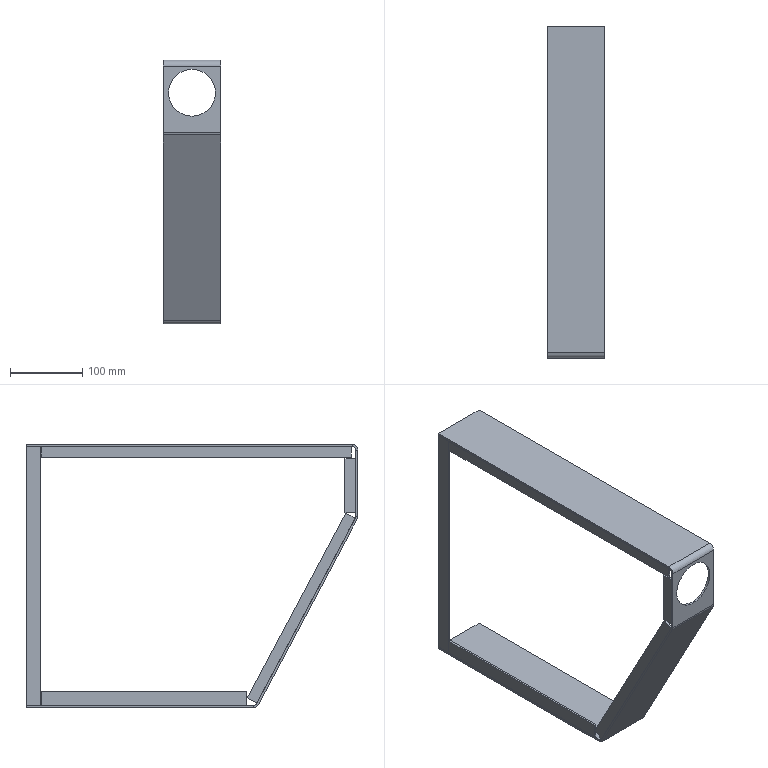Part | SolidWorks | features ICE 3, FlatPattern 1, SMBaseFlange 1, SheetMetal 1 | 6 solids | 62 faces | box 80 x 460 x 365 mm | volume 345434 mm3 | plane 54 | cylinder 8 | commonest cylinder face diameters 10 x3 16 x3 65 x2
STEP:
#1=CARTESIAN_POINT('',(40.,3.,-12.5));
#2=VERTEX_POINT('',#1);
#3=CARTESIAN_POINT('',(40.,3.,-77.5));
#4=VERTEX_POINT('',#3);
#5=CARTESIAN_POINT('',(40.,3.,-45.));
#6=DIRECTION('',(0.,-1.,0.));
#7=DIRECTION('',(0.,0.,-1.));
#8=AXIS2_PLACEMENT_3D('',#5,#6,#7);
#9=CIRCLE('',#8,32.5);
#10=EDGE_CURVE('',#2,#4,#9,.T.);
#11=ORIENTED_EDGE('',*,*,#10,.F.);
#12=CARTESIAN_POINT('',(40.,0.,-12.5));
#13=VERTEX_POINT('',#12);
#14=CARTESIAN_POINT('',(40.,10.,-12.5));
#15=DIRECTION('',(0.,-1.,0.));
#16=VECTOR('',#15,1000.);
#17=LINE('',#14,#16);
#18=EDGE_CURVE('',#2,#13,#17,.T.);
#19=ORIENTED_EDGE('',*,*,#18,.T.);
#20=CARTESIAN_POINT('',(40.,0.,-77.5));
#21=VERTEX_POINT('',#20);
#22=CARTESIAN_POINT('',(40.,0.,-45.));
#23=DIRECTION('',(0.,-1.,0.));
#24=DIRECTION('',(0.,0.,-1.));
#25=AXIS2_PLACEMENT_3D('',#22,#23,#24);
#26=CIRCLE('',#25,32.5);
#27=EDGE_CURVE('',#13,#21,#26,.T.);
#28=ORIENTED_EDGE('',*,*,#27,.T.);
#29=CARTESIAN_POINT('',(40.,10.,-77.5));
#30=DIRECTION('',(0.,-1.,0.));
#31=VECTOR('',#30,1000.);
#32=LINE('',#29,#31);
#33=EDGE_CURVE('',#4,#21,#32,.T.);
#34=ORIENTED_EDGE('',*,*,#33,.F.);
#35=EDGE_LOOP('',(#11,#19,#28,#34));
#36=FACE_OUTER_BOUND('',#35,.T.);
#37=CARTESIAN_POINT('',(40.,10.,-45.));
#38=DIRECTION('',(0.,-1.,0.));
#39=DIRECTION('',(0.,0.,-1.));
#40=AXIS2_PLACEMENT_3D('',#37,#38,#39);
#41=CYLINDRICAL_SURFACE('',#40,32.5);
#42=ADVANCED_FACE('',(#36),#41,.F.);
#43=CARTESIAN_POINT('',(80.,137.743,-360.756));
#44=VERTEX_POINT('',#43);
#45=CARTESIAN_POINT('',(80.,140.392,-359.347));
#46=VERTEX_POINT('',#45);
#47=CARTESIAN_POINT('',(80.,137.743,-360.756));
#48=DIRECTION('',(0.,0.8829,0.4695));
#49=VECTOR('',#48,1000.);
#50=LINE('',#47,#49);
#51=EDGE_CURVE('',#44,#46,#50,.T.);
#52=ORIENTED_EDGE('',*,*,#51,.F.);
#53=CARTESIAN_POINT('',(80.,144.807,-365.));
#54=VERTEX_POINT('',#53);
#55=CARTESIAN_POINT('',(80.,144.807,-357.));
#56=DIRECTION('',(-1.,0.,0.));
#57=DIRECTION('',(0.,0.,-1.));
#58=AXIS2_PLACEMENT_3D('',#55,#56,#57);
#59=CIRCLE('',#58,8.);
#60=EDGE_CURVE('',#54,#44,#59,.T.);
#61=ORIENTED_EDGE('',*,*,#60,.F.);
#62=CARTESIAN_POINT('',(80.,144.807,-362.));
#63=VERTEX_POINT('',#62);
#64=CARTESIAN_POINT('',(80.,144.807,-362.));
#65=DIRECTION('',(0.,0.,-1.));
#66=VECTOR('',#65,1000.);
#67=LINE('',#64,#66);
#68=EDGE_CURVE('',#63,#54,#67,.T.);
#69=ORIENTED_EDGE('',*,*,#68,.F.);
#70=CARTESIAN_POINT('',(80.,144.807,-357.));
#71=DIRECTION('',(-1.,0.,0.));
#72=DIRECTION('',(0.,0.,-1.));
#73=AXIS2_PLACEMENT_3D('',#70,#71,#72);
#74=CIRCLE('',#73,5.);
#75=EDGE_CURVE('',#63,#46,#74,.T.);
#76=ORIENTED_EDGE('',*,*,#75,.T.);
#77=EDGE_LOOP('',(#52,#61,#69,#76));
#78=FACE_OUTER_BOUND('',#77,.T.);
#79=CARTESIAN_POINT('',(80.,137.743,-360.756));
#80=DIRECTION('',(1.,0.,0.));
#81=DIRECTION('',(0.,0.,-1.));
#82=AXIS2_PLACEMENT_3D('',#79,#80,#81);
#83=PLANE('',#82);
#84=ADVANCED_FACE('',(#78),#83,.T.);
#85=CARTESIAN_POINT('',(80.,0.9364,-103.459));
#86=VERTEX_POINT('',#85);
#87=CARTESIAN_POINT('',(80.,0.,-101.698));
#88=DIRECTION('',(0.,-0.4695,0.8829));
#89=VECTOR('',#88,1000.);
#90=LINE('',#87,#89);
#91=EDGE_CURVE('',#44,#86,#90,.T.);
#92=ORIENTED_EDGE('',*,*,#91,.F.);
#93=ORIENTED_EDGE('',*,*,#51,.T.);
#94=CARTESIAN_POINT('',(80.,3.585,-102.051));
#95=VERTEX_POINT('',#94);
#96=CARTESIAN_POINT('',(80.,2.649,-100.29));
#97=DIRECTION('',(0.,-0.4695,0.8829));
#98=VECTOR('',#97,1000.);
#99=LINE('',#96,#98);
#100=EDGE_CURVE('',#46,#95,#99,.T.);
#101=ORIENTED_EDGE('',*,*,#100,.T.);
#102=CARTESIAN_POINT('',(80.,3.585,-102.051));
#103=DIRECTION('',(0.,-0.8829,-0.4695));
#104=VECTOR('',#103,1000.);
#105=LINE('',#102,#104);
#106=EDGE_CURVE('',#95,#86,#105,.T.);
#107=ORIENTED_EDGE('',*,*,#106,.T.);
#108=EDGE_LOOP('',(#92,#93,#101,#107));
#109=FACE_OUTER_BOUND('',#108,.T.);
#110=CARTESIAN_POINT('',(80.,144.807,-362.));
#111=DIRECTION('',(1.,0.,0.));
#112=DIRECTION('',(0.,0.,-1.));
#113=AXIS2_PLACEMENT_3D('',#110,#111,#112);
#114=PLANE('',#113);
#115=ADVANCED_FACE('',(#109),#114,.T.);
#116=CARTESIAN_POINT('',(0.,144.807,-365.));
#117=VERTEX_POINT('',#116);
#118=CARTESIAN_POINT('',(0.,144.807,-362.));
#119=VERTEX_POINT('',#118);
#120=CARTESIAN_POINT('',(0.,144.807,-365.));
#121=DIRECTION('',(0.,0.,1.));
#122=VECTOR('',#121,1000.);
#123=LINE('',#120,#122);
#124=EDGE_CURVE('',#117,#119,#123,.T.);
#125=ORIENTED_EDGE('',*,*,#124,.F.);
#126=CARTESIAN_POINT('',(0.,137.743,-360.756));
#127=VERTEX_POINT('',#126);
#128=CARTESIAN_POINT('',(0.,144.807,-357.));
#129=DIRECTION('',(-1.,0.,0.));
#130=DIRECTION('',(0.,0.,-1.));
#131=AXIS2_PLACEMENT_3D('',#128,#129,#130);
#132=CIRCLE('',#131,8.);
#133=EDGE_CURVE('',#117,#127,#132,.T.);
#134=ORIENTED_EDGE('',*,*,#133,.T.);
#135=CARTESIAN_POINT('',(0.,140.392,-359.347));
#136=VERTEX_POINT('',#135);
#137=CARTESIAN_POINT('',(0.,140.392,-359.347));
#138=DIRECTION('',(0.,-0.8829,-0.4695));
#139=VECTOR('',#138,1000.);
#140=LINE('',#137,#139);
#141=EDGE_CURVE('',#136,#127,#140,.T.);
#142=ORIENTED_EDGE('',*,*,#141,.F.);
#143=CARTESIAN_POINT('',(0.,144.807,-357.));
#144=DIRECTION('',(-1.,0.,0.));
#145=DIRECTION('',(0.,0.,-1.));
#146=AXIS2_PLACEMENT_3D('',#143,#144,#145);
#147=CIRCLE('',#146,5.);
#148=EDGE_CURVE('',#119,#136,#147,.T.);
#149=ORIENTED_EDGE('',*,*,#148,.F.);
#150=EDGE_LOOP('',(#125,#134,#142,#149));
#151=FACE_OUTER_BOUND('',#150,.T.);
#152=CARTESIAN_POINT('',(0.,144.807,-365.));
#153=DIRECTION('',(-1.,0.,0.));
#154=DIRECTION('',(0.,0.,1.));
#155=AXIS2_PLACEMENT_3D('',#152,#153,#154);
#156=PLANE('',#155);
#157=ADVANCED_FACE('',(#151),#156,.T.);
#158=CARTESIAN_POINT('',(0.,460.,-365.));
#159=VERTEX_POINT('',#158);
#160=CARTESIAN_POINT('',(0.,140.,-365.));
#161=DIRECTION('',(0.,-1.,0.));
#162=VECTOR('',#161,1000.);
#163=LINE('',#160,#162);
#164=EDGE_CURVE('',#159,#117,#163,.T.);
#165=ORIENTED_EDGE('',*,*,#164,.T.);
#166=ORIENTED_EDGE('',*,*,#124,.T.);
#167=CARTESIAN_POINT('',(0.,460.,-362.));
#168=VERTEX_POINT('',#167);
#169=CARTESIAN_POINT('',(0.,140.,-362.));
#170=DIRECTION('',(0.,-1.,0.));
#171=VECTOR('',#170,1000.);
#172=LINE('',#169,#171);
#173=EDGE_CURVE('',#168,#119,#172,.T.);
#174=ORIENTED_EDGE('',*,*,#173,.F.);
#175=CARTESIAN_POINT('',(0.,460.,-362.));
#176=DIRECTION('',(0.,0.,-1.));
#177=VECTOR('',#176,1000.);
#178=LINE('',#175,#177);
#179=EDGE_CURVE('',#168,#159,#178,.T.);
#180=ORIENTED_EDGE('',*,*,#179,.T.);
#181=EDGE_LOOP('',(#165,#166,#174,#180));
#182=FACE_OUTER_BOUND('',#181,.T.);
#183=CARTESIAN_POINT('',(0.,140.392,-359.347));
#184=DIRECTION('',(-1.,0.,0.));
#185=DIRECTION('',(0.,0.,1.));
#186=AXIS2_PLACEMENT_3D('',#183,#184,#185);
#187=PLANE('',#186);
#188=ADVANCED_FACE('',(#182),#187,.T.);
#189=CARTESIAN_POINT('',(80.,0.,-99.704));
#190=VERTEX_POINT('',#189);
#191=CARTESIAN_POINT('',(80.,3.,-99.704));
#192=VERTEX_POINT('',#191);
#193=CARTESIAN_POINT('',(80.,0.,-99.704));
#194=DIRECTION('',(0.,1.,0.));
#195=VECTOR('',#194,1000.);
#196=LINE('',#193,#195);
#197=EDGE_CURVE('',#190,#192,#196,.T.);
#198=ORIENTED_EDGE('',*,*,#197,.F.);
#199=CARTESIAN_POINT('',(80.,8.,-99.704));
#200=DIRECTION('',(-1.,0.,0.));
#201=DIRECTION('',(0.,0.,-1.));
#202=AXIS2_PLACEMENT_3D('',#199,#200,#201);
#203=CIRCLE('',#202,8.);
#204=EDGE_CURVE('',#86,#190,#203,.T.);
#205=ORIENTED_EDGE('',*,*,#204,.F.);
#206=ORIENTED_EDGE('',*,*,#106,.F.);
#207=CARTESIAN_POINT('',(80.,8.,-99.704));
#208=DIRECTION('',(-1.,0.,0.));
#209=DIRECTION('',(0.,0.,-1.));
#210=AXIS2_PLACEMENT_3D('',#207,#208,#209);
#211=CIRCLE('',#210,5.);
#212=EDGE_CURVE('',#95,#192,#211,.T.);
#213=ORIENTED_EDGE('',*,*,#212,.T.);
#214=EDGE_LOOP('',(#198,#205,#206,#213));
#215=FACE_OUTER_BOUND('',#214,.T.);
#216=CARTESIAN_POINT('',(80.,0.,-99.704));
#217=DIRECTION('',(1.,0.,0.));
#218=DIRECTION('',(0.,0.,-1.));
#219=AXIS2_PLACEMENT_3D('',#216,#217,#218);
#220=PLANE('',#219);
#221=ADVANCED_FACE('',(#215),#220,.T.);
#222=CARTESIAN_POINT('',(80.,0.,-8.));
#223=VERTEX_POINT('',#222);
#224=CARTESIAN_POINT('',(80.,0.,0.));
#225=DIRECTION('',(0.,0.,1.));
#226=VECTOR('',#225,1000.);
#227=LINE('',#224,#226);
#228=EDGE_CURVE('',#190,#223,#227,.T.);
#229=ORIENTED_EDGE('',*,*,#228,.F.);
#230=ORIENTED_EDGE('',*,*,#197,.T.);
#231=CARTESIAN_POINT('',(80.,3.,-8.));
#232=VERTEX_POINT('',#231);
#233=CARTESIAN_POINT('',(80.,3.,0.));
#234=DIRECTION('',(0.,0.,1.));
#235=VECTOR('',#234,1000.);
#236=LINE('',#233,#235);
#237=EDGE_CURVE('',#192,#232,#236,.T.);
#238=ORIENTED_EDGE('',*,*,#237,.T.);
#239=CARTESIAN_POINT('',(80.,3.,-8.));
#240=DIRECTION('',(0.,-1.,0.));
#241=VECTOR('',#240,1000.);
#242=LINE('',#239,#241);
#243=EDGE_CURVE('',#232,#223,#242,.T.);
#244=ORIENTED_EDGE('',*,*,#243,.T.);
#245=EDGE_LOOP('',(#229,#230,#238,#244));
#246=FACE_OUTER_BOUND('',#245,.T.);
#247=CARTESIAN_POINT('',(80.,3.585,-102.051));
#248=DIRECTION('',(1.,0.,0.));
#249=DIRECTION('',(0.,0.,-1.));
#250=AXIS2_PLACEMENT_3D('',#247,#248,#249);
#251=PLANE('',#250);
#252=ADVANCED_FACE('',(#246),#251,.T.);
#253=CARTESIAN_POINT('',(0.,0.9364,-103.459));
#254=VERTEX_POINT('',#253);
#255=CARTESIAN_POINT('',(0.,3.585,-102.051));
#256=VERTEX_POINT('',#255);
#257=CARTESIAN_POINT('',(0.,0.9364,-103.459));
#258=DIRECTION('',(0.,0.8829,0.4695));
#259=VECTOR('',#258,1000.);
#260=LINE('',#257,#259);
#261=EDGE_CURVE('',#254,#256,#260,.T.);
#262=ORIENTED_EDGE('',*,*,#261,.F.);
#263=CARTESIAN_POINT('',(0.,0.,-99.704));
#264=VERTEX_POINT('',#263);
#265=CARTESIAN_POINT('',(0.,8.,-99.704));
#266=DIRECTION('',(-1.,0.,0.));
#267=DIRECTION('',(0.,0.,-1.));
#268=AXIS2_PLACEMENT_3D('',#265,#266,#267);
#269=CIRCLE('',#268,8.);
#270=EDGE_CURVE('',#254,#264,#269,.T.);
#271=ORIENTED_EDGE('',*,*,#270,.T.);
#272=CARTESIAN_POINT('',(0.,3.,-99.704));
#273=VERTEX_POINT('',#272);
#274=CARTESIAN_POINT('',(0.,3.,-99.704));
#275=DIRECTION('',(0.,-1.,0.));
#276=VECTOR('',#275,1000.);
#277=LINE('',#274,#276);
#278=EDGE_CURVE('',#273,#264,#277,.T.);
#279=ORIENTED_EDGE('',*,*,#278,.F.);
#280=CARTESIAN_POINT('',(0.,8.,-99.704));
#281=DIRECTION('',(-1.,0.,0.));
#282=DIRECTION('',(0.,0.,-1.));
#283=AXIS2_PLACEMENT_3D('',#280,#281,#282);
#284=CIRCLE('',#283,5.);
#285=EDGE_CURVE('',#256,#273,#284,.T.);
#286=ORIENTED_EDGE('',*,*,#285,.F.);
#287=EDGE_LOOP('',(#262,#271,#279,#286));
#288=FACE_OUTER_BOUND('',#287,.T.);
#289=CARTESIAN_POINT('',(0.,0.9364,-103.459));
#290=DIRECTION('',(-1.,0.,0.));
#291=DIRECTION('',(0.,0.,1.));
#292=AXIS2_PLACEMENT_3D('',#289,#290,#291);
#293=PLANE('',#292);
#294=ADVANCED_FACE('',(#288),#293,.T.);
#295=CARTESIAN_POINT('',(0.,0.,-101.698));
#296=DIRECTION('',(0.,-0.4695,0.8829));
#297=VECTOR('',#296,1000.);
#298=LINE('',#295,#297);
#299=EDGE_CURVE('',#127,#254,#298,.T.);
#300=ORIENTED_EDGE('',*,*,#299,.T.);
#301=ORIENTED_EDGE('',*,*,#261,.T.);
#302=CARTESIAN_POINT('',(0.,2.649,-100.29));
#303=DIRECTION('',(0.,-0.4695,0.8829));
#304=VECTOR('',#303,1000.);
#305=LINE('',#302,#304);
#306=EDGE_CURVE('',#136,#256,#305,.T.);
#307=ORIENTED_EDGE('',*,*,#306,.F.);
#308=ORIENTED_EDGE('',*,*,#141,.T.);
#309=EDGE_LOOP('',(#300,#301,#307,#308));
#310=FACE_OUTER_BOUND('',#309,.T.);
#311=CARTESIAN_POINT('',(0.,3.,-99.704));
#312=DIRECTION('',(-1.,0.,0.));
#313=DIRECTION('',(0.,0.,1.));
#314=AXIS2_PLACEMENT_3D('',#311,#312,#313);
#315=PLANE('',#314);
#316=ADVANCED_FACE('',(#310),#315,.T.);
#317=CARTESIAN_POINT('',(80.,8.,0.));
#318=VERTEX_POINT('',#317);
#319=CARTESIAN_POINT('',(80.,8.,-3.));
#320=VERTEX_POINT('',#319);
#321=CARTESIAN_POINT('',(80.,8.,0.));
#322=DIRECTION('',(0.,0.,-1.));
#323=VECTOR('',#322,1000.);
#324=LINE('',#321,#323);
#325=EDGE_CURVE('',#318,#320,#324,.T.);
#326=ORIENTED_EDGE('',*,*,#325,.F.);
#327=CARTESIAN_POINT('',(80.,8.,-8.));
#328=DIRECTION('',(-1.,0.,0.));
#329=DIRECTION('',(0.,0.,-1.));
#330=AXIS2_PLACEMENT_3D('',#327,#328,#329);
#331=CIRCLE('',#330,8.);
#332=EDGE_CURVE('',#223,#318,#331,.T.);
#333=ORIENTED_EDGE('',*,*,#332,.F.);
#334=ORIENTED_EDGE('',*,*,#243,.F.);
#335=CARTESIAN_POINT('',(80.,8.,-8.));
#336=DIRECTION('',(-1.,0.,0.));
#337=DIRECTION('',(0.,0.,-1.));
#338=AXIS2_PLACEMENT_3D('',#335,#336,#337);
#339=CIRCLE('',#338,5.);
#340=EDGE_CURVE('',#232,#320,#339,.T.);
#341=ORIENTED_EDGE('',*,*,#340,.T.);
#342=EDGE_LOOP('',(#326,#333,#334,#341));
#343=FACE_OUTER_BOUND('',#342,.T.);
#344=CARTESIAN_POINT('',(80.,8.,0.));
#345=DIRECTION('',(1.,0.,0.));
#346=DIRECTION('',(0.,0.,-1.));
#347=AXIS2_PLACEMENT_3D('',#344,#345,#346);
#348=PLANE('',#347);
#349=ADVANCED_FACE('',(#343),#348,.T.);
#350=CARTESIAN_POINT('',(80.,460.,0.));
#351=VERTEX_POINT('',#350);
#352=CARTESIAN_POINT('',(80.,0.,0.));
#353=DIRECTION('',(0.,1.,0.));
#354=VECTOR('',#353,1000.);
#355=LINE('',#352,#354);
#356=EDGE_CURVE('',#318,#351,#355,.T.);
#357=ORIENTED_EDGE('',*,*,#356,.F.);
#358=ORIENTED_EDGE('',*,*,#325,.T.);
#359=CARTESIAN_POINT('',(80.,460.,-3.));
#360=VERTEX_POINT('',#359);
#361=CARTESIAN_POINT('',(80.,0.,-3.));
#362=DIRECTION('',(0.,1.,0.));
#363=VECTOR('',#362,1000.);
#364=LINE('',#361,#363);
#365=EDGE_CURVE('',#320,#360,#364,.T.);
#366=ORIENTED_EDGE('',*,*,#365,.T.);
#367=CARTESIAN_POINT('',(80.,460.,0.));
#368=DIRECTION('',(0.,0.,-1.));
#369=VECTOR('',#368,1000.);
#370=LINE('',#367,#369);
#371=EDGE_CURVE('',#351,#360,#370,.T.);
#372=ORIENTED_EDGE('',*,*,#371,.F.);
#373=EDGE_LOOP('',(#357,#358,#366,#372));
#374=FACE_OUTER_BOUND('',#373,.T.);
#375=CARTESIAN_POINT('',(80.,3.,-8.));
#376=DIRECTION('',(1.,0.,0.));
#377=DIRECTION('',(0.,0.,-1.));
#378=AXIS2_PLACEMENT_3D('',#375,#376,#377);
#379=PLANE('',#378);
#380=ADVANCED_FACE('',(#374),#379,.T.);
#381=CARTESIAN_POINT('',(0.,0.,-8.));
#382=VERTEX_POINT('',#381);
#383=CARTESIAN_POINT('',(0.,3.,-8.));
#384=VERTEX_POINT('',#383);
#385=CARTESIAN_POINT('',(0.,0.,-8.));
#386=DIRECTION('',(0.,1.,0.));
#387=VECTOR('',#386,1000.);
#388=LINE('',#385,#387);
#389=EDGE_CURVE('',#382,#384,#388,.T.);
#390=ORIENTED_EDGE('',*,*,#389,.F.);
#391=CARTESIAN_POINT('',(0.,8.,0.));
#392=VERTEX_POINT('',#391);
#393=CARTESIAN_POINT('',(0.,8.,-8.));
#394=DIRECTION('',(-1.,0.,0.));
#395=DIRECTION('',(0.,0.,-1.));
#396=AXIS2_PLACEMENT_3D('',#393,#394,#395);
#397=CIRCLE('',#396,8.);
#398=EDGE_CURVE('',#382,#392,#397,.T.);
#399=ORIENTED_EDGE('',*,*,#398,.T.);
#400=CARTESIAN_POINT('',(0.,8.,-3.));
#401=VERTEX_POINT('',#400);
#402=CARTESIAN_POINT('',(0.,8.,-3.));
#403=DIRECTION('',(0.,0.,1.));
#404=VECTOR('',#403,1000.);
#405=LINE('',#402,#404);
#406=EDGE_CURVE('',#401,#392,#405,.T.);
#407=ORIENTED_EDGE('',*,*,#406,.F.);
#408=CARTESIAN_POINT('',(0.,8.,-8.));
#409=DIRECTION('',(-1.,0.,0.));
#410=DIRECTION('',(0.,0.,-1.));
#411=AXIS2_PLACEMENT_3D('',#408,#409,#410);
#412=CIRCLE('',#411,5.);
#413=EDGE_CURVE('',#384,#401,#412,.T.);
#414=ORIENTED_EDGE('',*,*,#413,.F.);
#415=EDGE_LOOP('',(#390,#399,#407,#414));
#416=FACE_OUTER_BOUND('',#415,.T.);
#417=CARTESIAN_POINT('',(0.,0.,-8.));
#418=DIRECTION('',(-1.,0.,0.));
#419=DIRECTION('',(0.,0.,1.));
#420=AXIS2_PLACEMENT_3D('',#417,#418,#419);
#421=PLANE('',#420);
#422=ADVANCED_FACE('',(#416),#421,.T.);
#423=CARTESIAN_POINT('',(0.,0.,0.));
#424=DIRECTION('',(0.,0.,1.));
#425=VECTOR('',#424,1000.);
#426=LINE('',#423,#425);
#427=EDGE_CURVE('',#264,#382,#426,.T.);
#428=ORIENTED_EDGE('',*,*,#427,.T.);
#429=ORIENTED_EDGE('',*,*,#389,.T.);
#430=CARTESIAN_POINT('',(0.,3.,0.));
#431=DIRECTION('',(0.,0.,1.));
#432=VECTOR('',#431,1000.);
#433=LINE('',#430,#432);
#434=EDGE_CURVE('',#273,#384,#433,.T.);
#435=ORIENTED_EDGE('',*,*,#434,.F.);
#436=ORIENTED_EDGE('',*,*,#278,.T.);
#437=EDGE_LOOP('',(#428,#429,#435,#436));
#438=FACE_OUTER_BOUND('',#437,.T.);
#439=CARTESIAN_POINT('',(0.,8.,-3.));
#440=DIRECTION('',(-1.,0.,0.));
#441=DIRECTION('',(0.,0.,1.));
#442=AXIS2_PLACEMENT_3D('',#439,#440,#441);
#443=PLANE('',#442);
#444=ADVANCED_FACE('',(#438),#443,.T.);
#445=CARTESIAN_POINT('',(0.,460.,-3.));
#446=VERTEX_POINT('',#445);
#447=CARTESIAN_POINT('',(0.,0.,-3.));
#448=DIRECTION('',(0.,1.,0.));
#449=VECTOR('',#448,1000.);
#450=LINE('',#447,#449);
#451=EDGE_CURVE('',#401,#446,#450,.T.);
#452=ORIENTED_EDGE('',*,*,#451,.T.);
#453=CARTESIAN_POINT('',(80.,460.,-3.));
#454=DIRECTION('',(-1.,0.,0.));
#455=VECTOR('',#454,1000.);
#456=LINE('',#453,#455);
#457=EDGE_CURVE('',#360,#446,#456,.T.);
#458=ORIENTED_EDGE('',*,*,#457,.F.);
#459=ORIENTED_EDGE('',*,*,#365,.F.);
#460=CARTESIAN_POINT('',(80.,8.,-3.));
#461=DIRECTION('',(-1.,0.,0.));
#462=VECTOR('',#461,1000.);
#463=LINE('',#460,#462);
#464=EDGE_CURVE('',#320,#401,#463,.T.);
#465=ORIENTED_EDGE('',*,*,#464,.T.);
#466=EDGE_LOOP('',(#452,#458,#459,#465));
#467=FACE_OUTER_BOUND('',#466,.T.);
#468=CARTESIAN_POINT('',(80.,0.,-3.));
#469=DIRECTION('',(0.,0.,1.));
#470=DIRECTION('',(1.,0.,0.));
#471=AXIS2_PLACEMENT_3D('',#468,#469,#470);
#472=PLANE('',#471);
#473=ADVANCED_FACE('',(#467),#472,.F.);
#474=CARTESIAN_POINT('',(0.,460.,0.));
#475=VERTEX_POINT('',#474);
#476=CARTESIAN_POINT('',(0.,460.,0.));
#477=DIRECTION('',(0.,0.,-1.));
#478=VECTOR('',#477,1000.);
#479=LINE('',#476,#478);
#480=EDGE_CURVE('',#475,#446,#479,.T.);
#481=ORIENTED_EDGE('',*,*,#480,.F.);
#482=CARTESIAN_POINT('',(80.,460.,0.));
#483=DIRECTION('',(-1.,0.,0.));
#484=VECTOR('',#483,1000.);
#485=LINE('',#482,#484);
#486=EDGE_CURVE('',#351,#475,#485,.T.);
#487=ORIENTED_EDGE('',*,*,#486,.F.);
#488=ORIENTED_EDGE('',*,*,#371,.T.);
#489=ORIENTED_EDGE('',*,*,#457,.T.);
#490=EDGE_LOOP('',(#481,#487,#488,#489));
#491=FACE_OUTER_BOUND('',#490,.T.);
#492=CARTESIAN_POINT('',(80.,460.,0.));
#493=DIRECTION('',(0.,1.,0.));
#494=DIRECTION('',(0.,0.,1.));
#495=AXIS2_PLACEMENT_3D('',#492,#493,#494);
#496=PLANE('',#495);
#497=ADVANCED_FACE('',(#491),#496,.T.);
#498=CARTESIAN_POINT('',(0.,0.,0.));
#499=DIRECTION('',(0.,1.,0.));
#500=VECTOR('',#499,1000.);
#501=LINE('',#498,#500);
#502=EDGE_CURVE('',#392,#475,#501,.T.);
#503=ORIENTED_EDGE('',*,*,#502,.F.);
#504=CARTESIAN_POINT('',(80.,8.,0.));
#505=DIRECTION('',(-1.,0.,0.));
#506=VECTOR('',#505,1000.);
#507=LINE('',#504,#506);
#508=EDGE_CURVE('',#318,#392,#507,.T.);
#509=ORIENTED_EDGE('',*,*,#508,.F.);
#510=ORIENTED_EDGE('',*,*,#356,.T.);
#511=ORIENTED_EDGE('',*,*,#486,.T.);
#512=EDGE_LOOP('',(#503,#509,#510,#511));
#513=FACE_OUTER_BOUND('',#512,.T.);
#514=CARTESIAN_POINT('',(80.,0.,0.));
#515=DIRECTION('',(0.,0.,1.));
#516=DIRECTION('',(1.,0.,0.));
#517=AXIS2_PLACEMENT_3D('',#514,#515,#516);
#518=PLANE('',#517);
#519=ADVANCED_FACE('',(#513),#518,.T.);
#520=ORIENTED_EDGE('',*,*,#398,.F.);
#521=CARTESIAN_POINT('',(80.,0.,-8.));
#522=DIRECTION('',(-1.,0.,0.));
#523=VECTOR('',#522,1000.);
#524=LINE('',#521,#523);
#525=EDGE_CURVE('',#223,#382,#524,.T.);
#526=ORIENTED_EDGE('',*,*,#525,.F.);
#527=ORIENTED_EDGE('',*,*,#332,.T.);
#528=ORIENTED_EDGE('',*,*,#508,.T.);
#529=EDGE_LOOP('',(#520,#526,#527,#528));
#530=FACE_OUTER_BOUND('',#529,.T.);
#531=CARTESIAN_POINT('',(80.,8.,-8.));
#532=DIRECTION('',(-1.,0.,0.));
#533=DIRECTION('',(0.,0.,1.));
#534=AXIS2_PLACEMENT_3D('',#531,#532,#533);
#535=CYLINDRICAL_SURFACE('',#534,8.);
#536=ADVANCED_FACE('',(#530),#535,.T.);
#537=CARTESIAN_POINT('',(40.,0.,-45.));
#538=DIRECTION('',(0.,-1.,0.));
#539=DIRECTION('',(0.,0.,-1.));
#540=AXIS2_PLACEMENT_3D('',#537,#538,#539);
#541=CIRCLE('',#540,32.5);
#542=EDGE_CURVE('',#21,#13,#541,.T.);
#543=ORIENTED_EDGE('',*,*,#542,.F.);
#544=ORIENTED_EDGE('',*,*,#27,.F.);
#545=EDGE_LOOP('',(#543,#544));
#546=FACE_BOUND('',#545,.T.);
#547=ORIENTED_EDGE('',*,*,#427,.F.);
#548=CARTESIAN_POINT('',(80.,0.,-99.704));
#549=DIRECTION('',(-1.,0.,0.));
#550=VECTOR('',#549,1000.);
#551=LINE('',#548,#550);
#552=EDGE_CURVE('',#190,#264,#551,.T.);
#553=ORIENTED_EDGE('',*,*,#552,.F.);
#554=ORIENTED_EDGE('',*,*,#228,.T.);
#555=ORIENTED_EDGE('',*,*,#525,.T.);
#556=EDGE_LOOP('',(#547,#553,#554,#555));
#557=FACE_OUTER_BOUND('',#556,.T.);
#558=CARTESIAN_POINT('',(80.,0.,0.));
#559=DIRECTION('',(0.,-1.,0.));
#560=DIRECTION('',(0.,0.,-1.));
#561=AXIS2_PLACEMENT_3D('',#558,#559,#560);
#562=PLANE('',#561);
#563=ADVANCED_FACE('',(#546,#557),#562,.T.);
#564=ORIENTED_EDGE('',*,*,#270,.F.);
#565=CARTESIAN_POINT('',(80.,0.9364,-103.459));
#566=DIRECTION('',(-1.,0.,0.));
#567=VECTOR('',#566,1000.);
#568=LINE('',#565,#567);
#569=EDGE_CURVE('',#86,#254,#568,.T.);
#570=ORIENTED_EDGE('',*,*,#569,.F.);
#571=ORIENTED_EDGE('',*,*,#204,.T.);
#572=ORIENTED_EDGE('',*,*,#552,.T.);
#573=EDGE_LOOP('',(#564,#570,#571,#572));
#574=FACE_OUTER_BOUND('',#573,.T.);
#575=CARTESIAN_POINT('',(80.,8.,-99.704));
#576=DIRECTION('',(-1.,0.,0.));
#577=DIRECTION('',(0.,0.,1.));
#578=AXIS2_PLACEMENT_3D('',#575,#576,#577);
#579=CYLINDRICAL_SURFACE('',#578,8.);
#580=ADVANCED_FACE('',(#574),#579,.T.);
#581=ORIENTED_EDGE('',*,*,#299,.F.);
#582=CARTESIAN_POINT('',(80.,137.743,-360.756));
#583=DIRECTION('',(-1.,0.,0.));
#584=VECTOR('',#583,1000.);
#585=LINE('',#582,#584);
#586=EDGE_CURVE('',#44,#127,#585,.T.);
#587=ORIENTED_EDGE('',*,*,#586,.F.);
#588=ORIENTED_EDGE('',*,*,#91,.T.);
#589=ORIENTED_EDGE('',*,*,#569,.T.);
#590=EDGE_LOOP('',(#581,#587,#588,#589));
#591=FACE_OUTER_BOUND('',#590,.T.);
#592=CARTESIAN_POINT('',(80.,0.,-101.698));
#593=DIRECTION('',(0.,-0.8829,-0.4695));
#594=DIRECTION('',(0.,0.4695,-0.8829));
#595=AXIS2_PLACEMENT_3D('',#592,#593,#594);
#596=PLANE('',#595);
#597=ADVANCED_FACE('',(#591),#596,.T.);
#598=ORIENTED_EDGE('',*,*,#133,.F.);
#599=CARTESIAN_POINT('',(80.,144.807,-365.));
#600=DIRECTION('',(-1.,0.,0.));
#601=VECTOR('',#600,1000.);
#602=LINE('',#599,#601);
#603=EDGE_CURVE('',#54,#117,#602,.T.);
#604=ORIENTED_EDGE('',*,*,#603,.F.);
#605=ORIENTED_EDGE('',*,*,#60,.T.);
#606=ORIENTED_EDGE('',*,*,#586,.T.);
#607=EDGE_LOOP('',(#598,#604,#605,#606));
#608=FACE_OUTER_BOUND('',#607,.T.);
#609=CARTESIAN_POINT('',(80.,144.807,-357.));
#610=DIRECTION('',(-1.,0.,0.));
#611=DIRECTION('',(0.,0.,1.));
#612=AXIS2_PLACEMENT_3D('',#609,#610,#611);
#613=CYLINDRICAL_SURFACE('',#612,8.);
#614=ADVANCED_FACE('',(#608),#613,.T.);
#615=ORIENTED_EDGE('',*,*,#164,.F.);
#616=CARTESIAN_POINT('',(80.,460.,-365.));
#617=VERTEX_POINT('',#616);
#618=CARTESIAN_POINT('',(80.,460.,-365.));
#619=DIRECTION('',(-1.,0.,0.));
#620=VECTOR('',#619,1000.);
#621=LINE('',#618,#620);
#622=EDGE_CURVE('',#617,#159,#621,.T.);
#623=ORIENTED_EDGE('',*,*,#622,.F.);
#624=CARTESIAN_POINT('',(80.,140.,-365.));
#625=DIRECTION('',(0.,-1.,0.));
#626=VECTOR('',#625,1000.);
#627=LINE('',#624,#626);
#628=EDGE_CURVE('',#617,#54,#627,.T.);
#629=ORIENTED_EDGE('',*,*,#628,.T.);
#630=ORIENTED_EDGE('',*,*,#603,.T.);
#631=EDGE_LOOP('',(#615,#623,#629,#630));
#632=FACE_OUTER_BOUND('',#631,.T.);
#633=CARTESIAN_POINT('',(80.,140.,-365.));
#634=DIRECTION('',(0.,0.,-1.));
#635=DIRECTION('',(-1.,0.,0.));
#636=AXIS2_PLACEMENT_3D('',#633,#634,#635);
#637=PLANE('',#636);
#638=ADVANCED_FACE('',(#632),#637,.T.);
#639=ORIENTED_EDGE('',*,*,#179,.F.);
#640=CARTESIAN_POINT('',(80.,460.,-362.));
#641=VERTEX_POINT('',#640);
#642=CARTESIAN_POINT('',(80.,460.,-362.));
#643=DIRECTION('',(-1.,0.,0.));
#644=VECTOR('',#643,1000.);
#645=LINE('',#642,#644);
#646=EDGE_CURVE('',#641,#168,#645,.T.);
#647=ORIENTED_EDGE('',*,*,#646,.F.);
#648=CARTESIAN_POINT('',(80.,460.,-362.));
#649=DIRECTION('',(0.,0.,-1.));
#650=VECTOR('',#649,1000.);
#651=LINE('',#648,#650);
#652=EDGE_CURVE('',#641,#617,#651,.T.);
#653=ORIENTED_EDGE('',*,*,#652,.T.);
#654=ORIENTED_EDGE('',*,*,#622,.T.);
#655=EDGE_LOOP('',(#639,#647,#653,#654));
#656=FACE_OUTER_BOUND('',#655,.T.);
#657=CARTESIAN_POINT('',(80.,460.,-362.));
#658=DIRECTION('',(0.,1.,0.));
#659=DIRECTION('',(0.,0.,1.));
#660=AXIS2_PLACEMENT_3D('',#657,#658,#659);
#661=PLANE('',#660);
#662=ADVANCED_FACE('',(#656),#661,.T.);
#663=ORIENTED_EDGE('',*,*,#173,.T.);
#664=CARTESIAN_POINT('',(80.,144.807,-362.));
#665=DIRECTION('',(-1.,0.,0.));
#666=VECTOR('',#665,1000.);
#667=LINE('',#664,#666);
#668=EDGE_CURVE('',#63,#119,#667,.T.);
#669=ORIENTED_EDGE('',*,*,#668,.F.);
#670=CARTESIAN_POINT('',(80.,140.,-362.));
#671=DIRECTION('',(0.,-1.,0.));
#672=VECTOR('',#671,1000.);
#673=LINE('',#670,#672);
#674=EDGE_CURVE('',#641,#63,#673,.T.);
#675=ORIENTED_EDGE('',*,*,#674,.F.);
#676=ORIENTED_EDGE('',*,*,#646,.T.);
#677=EDGE_LOOP('',(#663,#669,#675,#676));
#678=FACE_OUTER_BOUND('',#677,.T.);
#679=CARTESIAN_POINT('',(80.,140.,-362.));
#680=DIRECTION('',(0.,0.,-1.));
#681=DIRECTION('',(-1.,0.,0.));
#682=AXIS2_PLACEMENT_3D('',#679,#680,#681);
#683=PLANE('',#682);
#684=ADVANCED_FACE('',(#678),#683,.F.);
#685=ORIENTED_EDGE('',*,*,#148,.T.);
#686=CARTESIAN_POINT('',(80.,140.392,-359.347));
#687=DIRECTION('',(-1.,0.,0.));
#688=VECTOR('',#687,1000.);
#689=LINE('',#686,#688);
#690=EDGE_CURVE('',#46,#136,#689,.T.);
#691=ORIENTED_EDGE('',*,*,#690,.F.);
#692=ORIENTED_EDGE('',*,*,#75,.F.);
#693=ORIENTED_EDGE('',*,*,#668,.T.);
#694=EDGE_LOOP('',(#685,#691,#692,#693));
#695=FACE_OUTER_BOUND('',#694,.T.);
#696=CARTESIAN_POINT('',(80.,144.807,-357.));
#697=DIRECTION('',(-1.,0.,0.));
#698=DIRECTION('',(0.,0.,1.));
#699=AXIS2_PLACEMENT_3D('',#696,#697,#698);
#700=CYLINDRICAL_SURFACE('',#699,5.);
#701=ADVANCED_FACE('',(#695),#700,.F.);
#702=ORIENTED_EDGE('',*,*,#306,.T.);
#703=CARTESIAN_POINT('',(80.,3.585,-102.051));
#704=DIRECTION('',(-1.,0.,0.));
#705=VECTOR('',#704,1000.);
#706=LINE('',#703,#705);
#707=EDGE_CURVE('',#95,#256,#706,.T.);
#708=ORIENTED_EDGE('',*,*,#707,.F.);
#709=ORIENTED_EDGE('',*,*,#100,.F.);
#710=ORIENTED_EDGE('',*,*,#690,.T.);
#711=EDGE_LOOP('',(#702,#708,#709,#710));
#712=FACE_OUTER_BOUND('',#711,.T.);
#713=CARTESIAN_POINT('',(80.,2.649,-100.29));
#714=DIRECTION('',(0.,-0.8829,-0.4695));
#715=DIRECTION('',(0.,0.4695,-0.8829));
#716=AXIS2_PLACEMENT_3D('',#713,#714,#715);
#717=PLANE('',#716);
#718=ADVANCED_FACE('',(#712),#717,.F.);
#719=ORIENTED_EDGE('',*,*,#285,.T.);
#720=CARTESIAN_POINT('',(80.,3.,-99.704));
#721=DIRECTION('',(-1.,0.,0.));
#722=VECTOR('',#721,1000.);
#723=LINE('',#720,#722);
#724=EDGE_CURVE('',#192,#273,#723,.T.);
#725=ORIENTED_EDGE('',*,*,#724,.F.);
#726=ORIENTED_EDGE('',*,*,#212,.F.);
#727=ORIENTED_EDGE('',*,*,#707,.T.);
#728=EDGE_LOOP('',(#719,#725,#726,#727));
#729=FACE_OUTER_BOUND('',#728,.T.);
#730=CARTESIAN_POINT('',(80.,8.,-99.704));
#731=DIRECTION('',(-1.,0.,0.));
#732=DIRECTION('',(0.,0.,1.));
#733=AXIS2_PLACEMENT_3D('',#730,#731,#732);
#734=CYLINDRICAL_SURFACE('',#733,5.);
#735=ADVANCED_FACE('',(#729),#734,.F.);
#736=CARTESIAN_POINT('',(40.,3.,-45.));
#737=DIRECTION('',(0.,-1.,0.));
#738=DIRECTION('',(0.,0.,-1.));
#739=AXIS2_PLACEMENT_3D('',#736,#737,#738);
#740=CIRCLE('',#739,32.5);
#741=EDGE_CURVE('',#4,#2,#740,.T.);
#742=ORIENTED_EDGE('',*,*,#741,.T.);
#743=ORIENTED_EDGE('',*,*,#10,.T.);
#744=EDGE_LOOP('',(#742,#743));
#745=FACE_BOUND('',#744,.T.);
#746=ORIENTED_EDGE('',*,*,#434,.T.);
#747=CARTESIAN_POINT('',(80.,3.,-8.));
#748=DIRECTION('',(-1.,0.,0.));
#749=VECTOR('',#748,1000.);
#750=LINE('',#747,#749);
#751=EDGE_CURVE('',#232,#384,#750,.T.);
#752=ORIENTED_EDGE('',*,*,#751,.F.);
#753=ORIENTED_EDGE('',*,*,#237,.F.);
#754=ORIENTED_EDGE('',*,*,#724,.T.);
#755=EDGE_LOOP('',(#746,#752,#753,#754));
#756=FACE_OUTER_BOUND('',#755,.T.);
#757=CARTESIAN_POINT('',(80.,3.,0.));
#758=DIRECTION('',(0.,-1.,0.));
#759=DIRECTION('',(0.,0.,-1.));
#760=AXIS2_PLACEMENT_3D('',#757,#758,#759);
#761=PLANE('',#760);
#762=ADVANCED_FACE('',(#745,#756),#761,.F.);
#763=ORIENTED_EDGE('',*,*,#413,.T.);
#764=ORIENTED_EDGE('',*,*,#464,.F.);
#765=ORIENTED_EDGE('',*,*,#340,.F.);
#766=ORIENTED_EDGE('',*,*,#751,.T.);
#767=EDGE_LOOP('',(#763,#764,#765,#766));
#768=FACE_OUTER_BOUND('',#767,.T.);
#769=CARTESIAN_POINT('',(80.,8.,-8.));
#770=DIRECTION('',(-1.,0.,0.));
#771=DIRECTION('',(0.,0.,1.));
#772=AXIS2_PLACEMENT_3D('',#769,#770,#771);
#773=CYLINDRICAL_SURFACE('',#772,5.);
#774=ADVANCED_FACE('',(#768),#773,.F.);
#775=ORIENTED_EDGE('',*,*,#674,.T.);
#776=ORIENTED_EDGE('',*,*,#68,.T.);
#777=ORIENTED_EDGE('',*,*,#628,.F.);
#778=ORIENTED_EDGE('',*,*,#652,.F.);
#779=EDGE_LOOP('',(#775,#776,#777,#778));
#780=FACE_OUTER_BOUND('',#779,.T.);
#781=CARTESIAN_POINT('',(80.,8.,-8.));
#782=DIRECTION('',(1.,0.,0.));
#783=DIRECTION('',(0.,0.,-1.));
#784=AXIS2_PLACEMENT_3D('',#781,#782,#783);
#785=PLANE('',#784);
#786=ADVANCED_FACE('',(#780),#785,.T.);
#787=ORIENTED_EDGE('',*,*,#451,.F.);
#788=ORIENTED_EDGE('',*,*,#406,.T.);
#789=ORIENTED_EDGE('',*,*,#502,.T.);
#790=ORIENTED_EDGE('',*,*,#480,.T.);
#791=EDGE_LOOP('',(#787,#788,#789,#790));
#792=FACE_OUTER_BOUND('',#791,.T.);
#793=CARTESIAN_POINT('',(0.,8.,-8.));
#794=DIRECTION('',(1.,0.,0.));
#795=DIRECTION('',(0.,0.,-1.));
#796=AXIS2_PLACEMENT_3D('',#793,#794,#795);
#797=PLANE('',#796);
#798=ADVANCED_FACE('',(#792),#797,.F.);
#799=ORIENTED_EDGE('',*,*,#18,.F.);
#800=ORIENTED_EDGE('',*,*,#741,.F.);
#801=ORIENTED_EDGE('',*,*,#33,.T.);
#802=ORIENTED_EDGE('',*,*,#542,.T.);
#803=EDGE_LOOP('',(#799,#800,#801,#802));
#804=FACE_OUTER_BOUND('',#803,.T.);
#805=CARTESIAN_POINT('',(40.,10.,-45.));
#806=DIRECTION('',(0.,-1.,0.));
#807=DIRECTION('',(0.,0.,-1.));
#808=AXIS2_PLACEMENT_3D('',#805,#806,#807);
#809=CYLINDRICAL_SURFACE('',#808,32.5);
#810=ADVANCED_FACE('',(#804),#809,.F.);
#811=CLOSED_SHELL('',(#42,#84,#115,#157,#188,#221,#252,#294,#316,#349,#380,#422,#444,#473,#497,#519,#536,#563,#580,#597,#614,#638,#662,#684,#701,#718,#735,#762,#774,#786,#798,#810));
#812=MANIFOLD_SOLID_BREP('',#811);
#813=CARTESIAN_POINT('',(0.,439.,-3.));
#814=VERTEX_POINT('',#813);
#815=CARTESIAN_POINT('',(0.,9.,-3.));
#816=VERTEX_POINT('',#815);
#817=CARTESIAN_POINT('',(0.,439.,-3.));
#818=DIRECTION('',(0.,-1.,0.));
#819=VECTOR('',#818,1000.);
#820=LINE('',#817,#819);
#821=EDGE_CURVE('',#814,#816,#820,.T.);
#822=ORIENTED_EDGE('',*,*,#821,.T.);
#823=CARTESIAN_POINT('',(3.,9.,-3.));
#824=VERTEX_POINT('',#823);
#825=CARTESIAN_POINT('',(3.,9.,-3.));
#826=DIRECTION('',(-1.,0.,0.));
#827=VECTOR('',#826,1000.);
#828=LINE('',#825,#827);
#829=EDGE_CURVE('',#824,#816,#828,.T.);
#830=ORIENTED_EDGE('',*,*,#829,.F.);
#831=CARTESIAN_POINT('',(3.,439.,-3.));
#832=VERTEX_POINT('',#831);
#833=CARTESIAN_POINT('',(3.,439.,-3.));
#834=DIRECTION('',(0.,-1.,0.));
#835=VECTOR('',#834,1000.);
#836=LINE('',#833,#835);
#837=EDGE_CURVE('',#832,#824,#836,.T.);
#838=ORIENTED_EDGE('',*,*,#837,.F.);
#839=CARTESIAN_POINT('',(3.,439.,-3.));
#840=DIRECTION('',(-1.,0.,0.));
#841=VECTOR('',#840,1000.);
#842=LINE('',#839,#841);
#843=EDGE_CURVE('',#832,#814,#842,.T.);
#844=ORIENTED_EDGE('',*,*,#843,.T.);
#845=EDGE_LOOP('',(#822,#830,#838,#844));
#846=FACE_OUTER_BOUND('',#845,.T.);
#847=CARTESIAN_POINT('',(3.,439.,-3.));
#848=DIRECTION('',(0.,0.,-1.));
#849=DIRECTION('',(0.,1.,0.));
#850=AXIS2_PLACEMENT_3D('',#847,#848,#849);
#851=PLANE('',#850);
#852=ADVANCED_FACE('',(#846),#851,.F.);
#853=CARTESIAN_POINT('',(0.,9.,-18.));
#854=VERTEX_POINT('',#853);
#855=CARTESIAN_POINT('',(0.,9.,-3.));
#856=DIRECTION('',(0.,0.,-1.));
#857=VECTOR('',#856,1000.);
#858=LINE('',#855,#857);
#859=EDGE_CURVE('',#816,#854,#858,.T.);
#860=ORIENTED_EDGE('',*,*,#859,.T.);
#861=CARTESIAN_POINT('',(3.,9.,-18.));
#862=VERTEX_POINT('',#861);
#863=CARTESIAN_POINT('',(3.,9.,-18.));
#864=DIRECTION('',(-1.,0.,0.));
#865=VECTOR('',#864,1000.);
#866=LINE('',#863,#865);
#867=EDGE_CURVE('',#862,#854,#866,.T.);
#868=ORIENTED_EDGE('',*,*,#867,.F.);
#869=CARTESIAN_POINT('',(3.,9.,-3.));
#870=DIRECTION('',(0.,0.,-1.));
#871=VECTOR('',#870,1000.);
#872=LINE('',#869,#871);
#873=EDGE_CURVE('',#824,#862,#872,.T.);
#874=ORIENTED_EDGE('',*,*,#873,.F.);
#875=ORIENTED_EDGE('',*,*,#829,.T.);
#876=EDGE_LOOP('',(#860,#868,#874,#875));
#877=FACE_OUTER_BOUND('',#876,.T.);
#878=CARTESIAN_POINT('',(3.,9.,-3.));
#879=DIRECTION('',(0.,1.,0.));
#880=DIRECTION('',(0.,0.,1.));
#881=AXIS2_PLACEMENT_3D('',#878,#879,#880);
#882=PLANE('',#881);
#883=ADVANCED_FACE('',(#877),#882,.F.);
#884=CARTESIAN_POINT('',(0.,439.,-18.));
#885=VERTEX_POINT('',#884);
#886=CARTESIAN_POINT('',(0.,439.,-18.));
#887=DIRECTION('',(0.,1.,0.));
#888=VECTOR('',#887,1000.);
#889=LINE('',#886,#888);
#890=EDGE_CURVE('',#854,#885,#889,.T.);
#891=ORIENTED_EDGE('',*,*,#890,.T.);
#892=CARTESIAN_POINT('',(3.,439.,-18.));
#893=VERTEX_POINT('',#892);
#894=CARTESIAN_POINT('',(3.,439.,-18.));
#895=DIRECTION('',(-1.,0.,0.));
#896=VECTOR('',#895,1000.);
#897=LINE('',#894,#896);
#898=EDGE_CURVE('',#893,#885,#897,.T.);
#899=ORIENTED_EDGE('',*,*,#898,.F.);
#900=CARTESIAN_POINT('',(3.,439.,-18.));
#901=DIRECTION('',(0.,1.,0.));
#902=VECTOR('',#901,1000.);
#903=LINE('',#900,#902);
#904=EDGE_CURVE('',#862,#893,#903,.T.);
#905=ORIENTED_EDGE('',*,*,#904,.F.);
#906=ORIENTED_EDGE('',*,*,#867,.T.);
#907=EDGE_LOOP('',(#891,#899,#905,#906));
#908=FACE_OUTER_BOUND('',#907,.T.);
#909=CARTESIAN_POINT('',(3.,439.,-18.));
#910=DIRECTION('',(0.,0.,1.));
#911=DIRECTION('',(0.,-1.,0.));
#912=AXIS2_PLACEMENT_3D('',#909,#910,#911);
#913=PLANE('',#912);
#914=ADVANCED_FACE('',(#908),#913,.F.);
#915=CARTESIAN_POINT('',(0.,439.,-3.));
#916=DIRECTION('',(0.,0.,1.));
#917=VECTOR('',#916,1000.);
#918=LINE('',#915,#917);
#919=EDGE_CURVE('',#885,#814,#918,.T.);
#920=ORIENTED_EDGE('',*,*,#919,.T.);
#921=ORIENTED_EDGE('',*,*,#843,.F.);
#922=CARTESIAN_POINT('',(3.,439.,-3.));
#923=DIRECTION('',(0.,0.,1.));
#924=VECTOR('',#923,1000.);
#925=LINE('',#922,#924);
#926=EDGE_CURVE('',#893,#832,#925,.T.);
#927=ORIENTED_EDGE('',*,*,#926,.F.);
#928=ORIENTED_EDGE('',*,*,#898,.T.);
#929=EDGE_LOOP('',(#920,#921,#927,#928));
#930=FACE_OUTER_BOUND('',#929,.T.);
#931=CARTESIAN_POINT('',(3.,439.,-3.));
#932=DIRECTION('',(0.,-1.,0.));
#933=DIRECTION('',(0.,0.,-1.));
#934=AXIS2_PLACEMENT_3D('',#931,#932,#933);
#935=PLANE('',#934);
#936=ADVANCED_FACE('',(#930),#935,.F.);
#937=ORIENTED_EDGE('',*,*,#837,.T.);
#938=ORIENTED_EDGE('',*,*,#873,.T.);
#939=ORIENTED_EDGE('',*,*,#904,.T.);
#940=ORIENTED_EDGE('',*,*,#926,.T.);
#941=EDGE_LOOP('',(#937,#938,#939,#940));
#942=FACE_OUTER_BOUND('',#941,.T.);
#943=CARTESIAN_POINT('',(3.,0.,0.));
#944=DIRECTION('',(1.,0.,0.));
#945=DIRECTION('',(0.,0.,-1.));
#946=AXIS2_PLACEMENT_3D('',#943,#944,#945);
#947=PLANE('',#946);
#948=ADVANCED_FACE('',(#942),#947,.T.);
#949=ORIENTED_EDGE('',*,*,#821,.F.);
#950=ORIENTED_EDGE('',*,*,#919,.F.);
#951=ORIENTED_EDGE('',*,*,#890,.F.);
#952=ORIENTED_EDGE('',*,*,#859,.F.);
#953=EDGE_LOOP('',(#949,#950,#951,#952));
#954=FACE_OUTER_BOUND('',#953,.T.);
#955=CARTESIAN_POINT('',(0.,0.,0.));
#956=DIRECTION('',(1.,0.,0.));
#957=DIRECTION('',(0.,0.,-1.));
#958=AXIS2_PLACEMENT_3D('',#955,#956,#957);
#959=PLANE('',#958);
#960=ADVANCED_FACE('',(#954),#959,.F.);
#961=CLOSED_SHELL('',(#852,#883,#914,#936,#948,#960));
#962=MANIFOLD_SOLID_BREP('',#961);
#963=CARTESIAN_POINT('',(0.,154.,-362.));
#964=VERTEX_POINT('',#963);
#965=CARTESIAN_POINT('',(0.,439.,-362.));
#966=VERTEX_POINT('',#965);
#967=CARTESIAN_POINT('',(0.,439.,-362.));
#968=DIRECTION('',(0.,1.,0.));
#969=VECTOR('',#968,1000.);
#970=LINE('',#967,#969);
#971=EDGE_CURVE('',#964,#966,#970,.T.);
#972=ORIENTED_EDGE('',*,*,#971,.T.);
#973=CARTESIAN_POINT('',(3.,439.,-362.));
#974=VERTEX_POINT('',#973);
#975=CARTESIAN_POINT('',(3.,439.,-362.));
#976=DIRECTION('',(-1.,0.,0.));
#977=VECTOR('',#976,1000.);
#978=LINE('',#975,#977);
#979=EDGE_CURVE('',#974,#966,#978,.T.);
#980=ORIENTED_EDGE('',*,*,#979,.F.);
#981=CARTESIAN_POINT('',(3.,154.,-362.));
#982=VERTEX_POINT('',#981);
#983=CARTESIAN_POINT('',(3.,439.,-362.));
#984=DIRECTION('',(0.,1.,0.));
#985=VECTOR('',#984,1000.);
#986=LINE('',#983,#985);
#987=EDGE_CURVE('',#982,#974,#986,.T.);
#988=ORIENTED_EDGE('',*,*,#987,.F.);
#989=CARTESIAN_POINT('',(3.,154.,-362.));
#990=DIRECTION('',(-1.,0.,0.));
#991=VECTOR('',#990,1000.);
#992=LINE('',#989,#991);
#993=EDGE_CURVE('',#982,#964,#992,.T.);
#994=ORIENTED_EDGE('',*,*,#993,.T.);
#995=EDGE_LOOP('',(#972,#980,#988,#994));
#996=FACE_OUTER_BOUND('',#995,.T.);
#997=CARTESIAN_POINT('',(3.,439.,-362.));
#998=DIRECTION('',(0.,0.,1.));
#999=DIRECTION('',(0.,-1.,0.));
#1000=AXIS2_PLACEMENT_3D('',#997,#998,#999);
#1001=PLANE('',#1000);
#1002=ADVANCED_FACE('',(#996),#1001,.F.);
#1003=CARTESIAN_POINT('',(0.,439.,-342.));
#1004=VERTEX_POINT('',#1003);
#1005=CARTESIAN_POINT('',(0.,439.,-362.));
#1006=DIRECTION('',(0.,0.,1.));
#1007=VECTOR('',#1006,1000.);
#1008=LINE('',#1005,#1007);
#1009=EDGE_CURVE('',#966,#1004,#1008,.T.);
#1010=ORIENTED_EDGE('',*,*,#1009,.T.);
#1011=CARTESIAN_POINT('',(3.,439.,-342.));
#1012=VERTEX_POINT('',#1011);
#1013=CARTESIAN_POINT('',(3.,439.,-342.));
#1014=DIRECTION('',(-1.,0.,0.));
#1015=VECTOR('',#1014,1000.);
#1016=LINE('',#1013,#1015);
#1017=EDGE_CURVE('',#1012,#1004,#1016,.T.);
#1018=ORIENTED_EDGE('',*,*,#1017,.F.);
#1019=CARTESIAN_POINT('',(3.,439.,-362.));
#1020=DIRECTION('',(0.,0.,1.));
#1021=VECTOR('',#1020,1000.);
#1022=LINE('',#1019,#1021);
#1023=EDGE_CURVE('',#974,#1012,#1022,.T.);
#1024=ORIENTED_EDGE('',*,*,#1023,.F.);
#1025=ORIENTED_EDGE('',*,*,#979,.T.);
#1026=EDGE_LOOP('',(#1010,#1018,#1024,#1025));
#1027=FACE_OUTER_BOUND('',#1026,.T.);
#1028=CARTESIAN_POINT('',(3.,439.,-362.));
#1029=DIRECTION('',(0.,-1.,0.));
#1030=DIRECTION('',(0.,0.,-1.));
#1031=AXIS2_PLACEMENT_3D('',#1028,#1029,#1030);
#1032=PLANE('',#1031);
#1033=ADVANCED_FACE('',(#1027),#1032,.F.);
#1034=CARTESIAN_POINT('',(0.,154.,-342.));
#1035=VERTEX_POINT('',#1034);
#1036=CARTESIAN_POINT('',(0.,439.,-342.));
#1037=DIRECTION('',(0.,-1.,0.));
#1038=VECTOR('',#1037,1000.);
#1039=LINE('',#1036,#1038);
#1040=EDGE_CURVE('',#1004,#1035,#1039,.T.);
#1041=ORIENTED_EDGE('',*,*,#1040,.T.);
#1042=CARTESIAN_POINT('',(3.,154.,-342.));
#1043=VERTEX_POINT('',#1042);
#1044=CARTESIAN_POINT('',(3.,154.,-342.));
#1045=DIRECTION('',(-1.,0.,0.));
#1046=VECTOR('',#1045,1000.);
#1047=LINE('',#1044,#1046);
#1048=EDGE_CURVE('',#1043,#1035,#1047,.T.);
#1049=ORIENTED_EDGE('',*,*,#1048,.F.);
#1050=CARTESIAN_POINT('',(3.,439.,-342.));
#1051=DIRECTION('',(0.,-1.,0.));
#1052=VECTOR('',#1051,1000.);
#1053=LINE('',#1050,#1052);
#1054=EDGE_CURVE('',#1012,#1043,#1053,.T.);
#1055=ORIENTED_EDGE('',*,*,#1054,.F.);
#1056=ORIENTED_EDGE('',*,*,#1017,.T.);
#1057=EDGE_LOOP('',(#1041,#1049,#1055,#1056));
#1058=FACE_OUTER_BOUND('',#1057,.T.);
#1059=CARTESIAN_POINT('',(3.,439.,-342.));
#1060=DIRECTION('',(0.,0.,-1.));
#1061=DIRECTION('',(0.,1.,0.));
#1062=AXIS2_PLACEMENT_3D('',#1059,#1060,#1061);
#1063=PLANE('',#1062);
#1064=ADVANCED_FACE('',(#1058),#1063,.F.);
#1065=CARTESIAN_POINT('',(0.,154.,-362.));
#1066=DIRECTION('',(0.,0.,-1.));
#1067=VECTOR('',#1066,1000.);
#1068=LINE('',#1065,#1067);
#1069=EDGE_CURVE('',#1035,#964,#1068,.T.);
#1070=ORIENTED_EDGE('',*,*,#1069,.T.);
#1071=ORIENTED_EDGE('',*,*,#993,.F.);
#1072=CARTESIAN_POINT('',(3.,154.,-362.));
#1073=DIRECTION('',(0.,0.,-1.));
#1074=VECTOR('',#1073,1000.);
#1075=LINE('',#1072,#1074);
#1076=EDGE_CURVE('',#1043,#982,#1075,.T.);
#1077=ORIENTED_EDGE('',*,*,#1076,.F.);
#1078=ORIENTED_EDGE('',*,*,#1048,.T.);
#1079=EDGE_LOOP('',(#1070,#1071,#1077,#1078));
#1080=FACE_OUTER_BOUND('',#1079,.T.);
#1081=CARTESIAN_POINT('',(3.,154.,-362.));
#1082=DIRECTION('',(0.,1.,0.));
#1083=DIRECTION('',(0.,0.,1.));
#1084=AXIS2_PLACEMENT_3D('',#1081,#1082,#1083);
#1085=PLANE('',#1084);
#1086=ADVANCED_FACE('',(#1080),#1085,.F.);
#1087=ORIENTED_EDGE('',*,*,#987,.T.);
#1088=ORIENTED_EDGE('',*,*,#1023,.T.);
#1089=ORIENTED_EDGE('',*,*,#1054,.T.);
#1090=ORIENTED_EDGE('',*,*,#1076,.T.);
#1091=EDGE_LOOP('',(#1087,#1088,#1089,#1090));
#1092=FACE_OUTER_BOUND('',#1091,.T.);
#1093=CARTESIAN_POINT('',(3.,0.,0.));
#1094=DIRECTION('',(-1.,0.,0.));
#1095=DIRECTION('',(0.,0.,1.));
#1096=AXIS2_PLACEMENT_3D('',#1093,#1094,#1095);
#1097=PLANE('',#1096);
#1098=ADVANCED_FACE('',(#1092),#1097,.F.);
#1099=ORIENTED_EDGE('',*,*,#971,.F.);
#1100=ORIENTED_EDGE('',*,*,#1069,.F.);
#1101=ORIENTED_EDGE('',*,*,#1040,.F.);
#1102=ORIENTED_EDGE('',*,*,#1009,.F.);
#1103=EDGE_LOOP('',(#1099,#1100,#1101,#1102));
#1104=FACE_OUTER_BOUND('',#1103,.T.);
#1105=CARTESIAN_POINT('',(0.,0.,0.));
#1106=DIRECTION('',(-1.,0.,0.));
#1107=DIRECTION('',(0.,0.,1.));
#1108=AXIS2_PLACEMENT_3D('',#1105,#1106,#1107);
#1109=PLANE('',#1108);
#1110=ADVANCED_FACE('',(#1104),#1109,.T.);
#1111=CLOSED_SHELL('',(#1002,#1033,#1064,#1086,#1098,#1110));
#1112=MANIFOLD_SOLID_BREP('',#1111);
#1113=CARTESIAN_POINT('',(0.,139.923,-358.464));
#1114=VERTEX_POINT('',#1113);
#1115=CARTESIAN_POINT('',(0.,3.776,-102.41));
#1116=VERTEX_POINT('',#1115);
#1117=CARTESIAN_POINT('',(0.,3.776,-102.41));
#1118=DIRECTION('',(0.,-0.4695,0.8829));
#1119=VECTOR('',#1118,1000.);
#1120=LINE('',#1117,#1119);
#1121=EDGE_CURVE('',#1114,#1116,#1120,.T.);
#1122=ORIENTED_EDGE('',*,*,#1121,.F.);
#1123=CARTESIAN_POINT('',(3.,139.923,-358.464));
#1124=VERTEX_POINT('',#1123);
#1125=CARTESIAN_POINT('',(3.,139.923,-358.464));
#1126=DIRECTION('',(-1.,0.,0.));
#1127=VECTOR('',#1126,1000.);
#1128=LINE('',#1125,#1127);
#1129=EDGE_CURVE('',#1124,#1114,#1128,.T.);
#1130=ORIENTED_EDGE('',*,*,#1129,.F.);
#1131=CARTESIAN_POINT('',(3.,3.776,-102.41));
#1132=VERTEX_POINT('',#1131);
#1133=CARTESIAN_POINT('',(3.,3.776,-102.41));
#1134=DIRECTION('',(0.,-0.4695,0.8829));
#1135=VECTOR('',#1134,1000.);
#1136=LINE('',#1133,#1135);
#1137=EDGE_CURVE('',#1124,#1132,#1136,.T.);
#1138=ORIENTED_EDGE('',*,*,#1137,.T.);
#1139=CARTESIAN_POINT('',(3.,3.776,-102.41));
#1140=DIRECTION('',(-1.,0.,0.));
#1141=VECTOR('',#1140,1000.);
#1142=LINE('',#1139,#1141);
#1143=EDGE_CURVE('',#1132,#1116,#1142,.T.);
#1144=ORIENTED_EDGE('',*,*,#1143,.T.);
#1145=EDGE_LOOP('',(#1122,#1130,#1138,#1144));
#1146=FACE_OUTER_BOUND('',#1145,.T.);
#1147=CARTESIAN_POINT('',(3.,3.776,-102.41));
#1148=DIRECTION('',(0.,-0.8829,-0.4695));
#1149=DIRECTION('',(0.,0.4695,-0.8829));
#1150=AXIS2_PLACEMENT_3D('',#1147,#1148,#1149);
#1151=PLANE('',#1150);
#1152=ADVANCED_FACE('',(#1146),#1151,.T.);
#1153=CARTESIAN_POINT('',(0.,153.167,-351.422));
#1154=VERTEX_POINT('',#1153);
#1155=CARTESIAN_POINT('',(0.,139.923,-358.464));
#1156=DIRECTION('',(0.,-0.8829,-0.4695));
#1157=VECTOR('',#1156,1000.);
#1158=LINE('',#1155,#1157);
#1159=EDGE_CURVE('',#1154,#1114,#1158,.T.);
#1160=ORIENTED_EDGE('',*,*,#1159,.F.);
#1161=CARTESIAN_POINT('',(3.,153.167,-351.422));
#1162=VERTEX_POINT('',#1161);
#1163=CARTESIAN_POINT('',(3.,153.167,-351.422));
#1164=DIRECTION('',(-1.,0.,0.));
#1165=VECTOR('',#1164,1000.);
#1166=LINE('',#1163,#1165);
#1167=EDGE_CURVE('',#1162,#1154,#1166,.T.);
#1168=ORIENTED_EDGE('',*,*,#1167,.F.);
#1169=CARTESIAN_POINT('',(3.,139.923,-358.464));
#1170=DIRECTION('',(0.,-0.8829,-0.4695));
#1171=VECTOR('',#1170,1000.);
#1172=LINE('',#1169,#1171);
#1173=EDGE_CURVE('',#1162,#1124,#1172,.T.);
#1174=ORIENTED_EDGE('',*,*,#1173,.T.);
#1175=ORIENTED_EDGE('',*,*,#1129,.T.);
#1176=EDGE_LOOP('',(#1160,#1168,#1174,#1175));
#1177=FACE_OUTER_BOUND('',#1176,.T.);
#1178=CARTESIAN_POINT('',(3.,139.923,-358.464));
#1179=DIRECTION('',(0.,0.4695,-0.8829));
#1180=DIRECTION('',(0.,0.8829,0.4695));
#1181=AXIS2_PLACEMENT_3D('',#1178,#1179,#1180);
#1182=PLANE('',#1181);
#1183=ADVANCED_FACE('',(#1177),#1182,.T.);
#1184=CARTESIAN_POINT('',(0.,17.02,-95.368));
#1185=VERTEX_POINT('',#1184);
#1186=CARTESIAN_POINT('',(0.,153.167,-351.422));
#1187=DIRECTION('',(0.,0.4695,-0.8829));
#1188=VECTOR('',#1187,1000.);
#1189=LINE('',#1186,#1188);
#1190=EDGE_CURVE('',#1185,#1154,#1189,.T.);
#1191=ORIENTED_EDGE('',*,*,#1190,.F.);
#1192=CARTESIAN_POINT('',(3.,17.02,-95.368));
#1193=VERTEX_POINT('',#1192);
#1194=CARTESIAN_POINT('',(3.,17.02,-95.368));
#1195=DIRECTION('',(-1.,0.,0.));
#1196=VECTOR('',#1195,1000.);
#1197=LINE('',#1194,#1196);
#1198=EDGE_CURVE('',#1193,#1185,#1197,.T.);
#1199=ORIENTED_EDGE('',*,*,#1198,.F.);
#1200=CARTESIAN_POINT('',(3.,153.167,-351.422));
#1201=DIRECTION('',(0.,0.4695,-0.8829));
#1202=VECTOR('',#1201,1000.);
#1203=LINE('',#1200,#1202);
#1204=EDGE_CURVE('',#1193,#1162,#1203,.T.);
#1205=ORIENTED_EDGE('',*,*,#1204,.T.);
#1206=ORIENTED_EDGE('',*,*,#1167,.T.);
#1207=EDGE_LOOP('',(#1191,#1199,#1205,#1206));
#1208=FACE_OUTER_BOUND('',#1207,.T.);
#1209=CARTESIAN_POINT('',(3.,153.167,-351.422));
#1210=DIRECTION('',(0.,0.8829,0.4695));
#1211=DIRECTION('',(0.,-0.4695,0.8829));
#1212=AXIS2_PLACEMENT_3D('',#1209,#1210,#1211);
#1213=PLANE('',#1212);
#1214=ADVANCED_FACE('',(#1208),#1213,.T.);
#1215=CARTESIAN_POINT('',(0.,17.02,-95.368));
#1216=DIRECTION('',(0.,0.8829,0.4695));
#1217=VECTOR('',#1216,1000.);
#1218=LINE('',#1215,#1217);
#1219=EDGE_CURVE('',#1116,#1185,#1218,.T.);
#1220=ORIENTED_EDGE('',*,*,#1219,.F.);
#1221=ORIENTED_EDGE('',*,*,#1143,.F.);
#1222=CARTESIAN_POINT('',(3.,17.02,-95.368));
#1223=DIRECTION('',(0.,0.8829,0.4695));
#1224=VECTOR('',#1223,1000.);
#1225=LINE('',#1222,#1224);
#1226=EDGE_CURVE('',#1132,#1193,#1225,.T.);
#1227=ORIENTED_EDGE('',*,*,#1226,.T.);
#1228=ORIENTED_EDGE('',*,*,#1198,.T.);
#1229=EDGE_LOOP('',(#1220,#1221,#1227,#1228));
#1230=FACE_OUTER_BOUND('',#1229,.T.);
#1231=CARTESIAN_POINT('',(3.,17.02,-95.368));
#1232=DIRECTION('',(0.,-0.4695,0.8829));
#1233=DIRECTION('',(0.,-0.8829,-0.4695));
#1234=AXIS2_PLACEMENT_3D('',#1231,#1232,#1233);
#1235=PLANE('',#1234);
#1236=ADVANCED_FACE('',(#1230),#1235,.T.);
#1237=ORIENTED_EDGE('',*,*,#1137,.F.);
#1238=ORIENTED_EDGE('',*,*,#1173,.F.);
#1239=ORIENTED_EDGE('',*,*,#1204,.F.);
#1240=ORIENTED_EDGE('',*,*,#1226,.F.);
#1241=EDGE_LOOP('',(#1237,#1238,#1239,#1240));
#1242=FACE_OUTER_BOUND('',#1241,.T.);
#1243=CARTESIAN_POINT('',(3.,0.,0.));
#1244=DIRECTION('',(1.,0.,0.));
#1245=DIRECTION('',(0.,0.,-1.));
#1246=AXIS2_PLACEMENT_3D('',#1243,#1244,#1245);
#1247=PLANE('',#1246);
#1248=ADVANCED_FACE('',(#1242),#1247,.T.);
#1249=ORIENTED_EDGE('',*,*,#1121,.T.);
#1250=ORIENTED_EDGE('',*,*,#1219,.T.);
#1251=ORIENTED_EDGE('',*,*,#1190,.T.);
#1252=ORIENTED_EDGE('',*,*,#1159,.T.);
#1253=EDGE_LOOP('',(#1249,#1250,#1251,#1252));
#1254=FACE_OUTER_BOUND('',#1253,.T.);
#1255=CARTESIAN_POINT('',(0.,0.,0.));
#1256=DIRECTION('',(1.,0.,0.));
#1257=DIRECTION('',(0.,0.,-1.));
#1258=AXIS2_PLACEMENT_3D('',#1255,#1256,#1257);
#1259=PLANE('',#1258);
#1260=ADVANCED_FACE('',(#1254),#1259,.F.);
#1261=CLOSED_SHELL('',(#1152,#1183,#1214,#1236,#1248,#1260));
#1262=MANIFOLD_SOLID_BREP('',#1261);
#1263=CARTESIAN_POINT('',(0.,3.,-95.));
#1264=VERTEX_POINT('',#1263);
#1265=CARTESIAN_POINT('',(0.,3.,-20.));
#1266=VERTEX_POINT('',#1265);
#1267=CARTESIAN_POINT('',(0.,3.,-20.));
#1268=DIRECTION('',(0.,0.,1.));
#1269=VECTOR('',#1268,1000.);
#1270=LINE('',#1267,#1269);
#1271=EDGE_CURVE('',#1264,#1266,#1270,.T.);
#1272=ORIENTED_EDGE('',*,*,#1271,.F.);
#1273=CARTESIAN_POINT('',(3.,3.,-95.));
#1274=VERTEX_POINT('',#1273);
#1275=CARTESIAN_POINT('',(3.,3.,-95.));
#1276=DIRECTION('',(-1.,0.,0.));
#1277=VECTOR('',#1276,1000.);
#1278=LINE('',#1275,#1277);
#1279=EDGE_CURVE('',#1274,#1264,#1278,.T.);
#1280=ORIENTED_EDGE('',*,*,#1279,.F.);
#1281=CARTESIAN_POINT('',(3.,3.,-20.));
#1282=VERTEX_POINT('',#1281);
#1283=CARTESIAN_POINT('',(3.,3.,-20.));
#1284=DIRECTION('',(0.,0.,1.));
#1285=VECTOR('',#1284,1000.);
#1286=LINE('',#1283,#1285);
#1287=EDGE_CURVE('',#1274,#1282,#1286,.T.);
#1288=ORIENTED_EDGE('',*,*,#1287,.T.);
#1289=CARTESIAN_POINT('',(3.,3.,-20.));
#1290=DIRECTION('',(-1.,0.,0.));
#1291=VECTOR('',#1290,1000.);
#1292=LINE('',#1289,#1291);
#1293=EDGE_CURVE('',#1282,#1266,#1292,.T.);
#1294=ORIENTED_EDGE('',*,*,#1293,.T.);
#1295=EDGE_LOOP('',(#1272,#1280,#1288,#1294));
#1296=FACE_OUTER_BOUND('',#1295,.T.);
#1297=CARTESIAN_POINT('',(3.,3.,-20.));
#1298=DIRECTION('',(0.,-1.,0.));
#1299=DIRECTION('',(0.,0.,-1.));
#1300=AXIS2_PLACEMENT_3D('',#1297,#1298,#1299);
#1301=PLANE('',#1300);
#1302=ADVANCED_FACE('',(#1296),#1301,.T.);
#1303=CARTESIAN_POINT('',(0.,18.,-95.));
#1304=VERTEX_POINT('',#1303);
#1305=CARTESIAN_POINT('',(0.,3.,-95.));
#1306=DIRECTION('',(0.,-1.,0.));
#1307=VECTOR('',#1306,1000.);
#1308=LINE('',#1305,#1307);
#1309=EDGE_CURVE('',#1304,#1264,#1308,.T.);
#1310=ORIENTED_EDGE('',*,*,#1309,.F.);
#1311=CARTESIAN_POINT('',(3.,18.,-95.));
#1312=VERTEX_POINT('',#1311);
#1313=CARTESIAN_POINT('',(3.,18.,-95.));
#1314=DIRECTION('',(-1.,0.,0.));
#1315=VECTOR('',#1314,1000.);
#1316=LINE('',#1313,#1315);
#1317=EDGE_CURVE('',#1312,#1304,#1316,.T.);
#1318=ORIENTED_EDGE('',*,*,#1317,.F.);
#1319=CARTESIAN_POINT('',(3.,3.,-95.));
#1320=DIRECTION('',(0.,-1.,0.));
#1321=VECTOR('',#1320,1000.);
#1322=LINE('',#1319,#1321);
#1323=EDGE_CURVE('',#1312,#1274,#1322,.T.);
#1324=ORIENTED_EDGE('',*,*,#1323,.T.);
#1325=ORIENTED_EDGE('',*,*,#1279,.T.);
#1326=EDGE_LOOP('',(#1310,#1318,#1324,#1325));
#1327=FACE_OUTER_BOUND('',#1326,.T.);
#1328=CARTESIAN_POINT('',(3.,3.,-95.));
#1329=DIRECTION('',(0.,0.,-1.));
#1330=DIRECTION('',(-1.,0.,0.));
#1331=AXIS2_PLACEMENT_3D('',#1328,#1329,#1330);
#1332=PLANE('',#1331);
#1333=ADVANCED_FACE('',(#1327),#1332,.T.);
#1334=CARTESIAN_POINT('',(0.,18.,-20.));
#1335=VERTEX_POINT('',#1334);
#1336=CARTESIAN_POINT('',(0.,18.,-95.));
#1337=DIRECTION('',(0.,0.,-1.));
#1338=VECTOR('',#1337,1000.);
#1339=LINE('',#1336,#1338);
#1340=EDGE_CURVE('',#1335,#1304,#1339,.T.);
#1341=ORIENTED_EDGE('',*,*,#1340,.F.);
#1342=CARTESIAN_POINT('',(3.,18.,-20.));
#1343=VERTEX_POINT('',#1342);
#1344=CARTESIAN_POINT('',(3.,18.,-20.));
#1345=DIRECTION('',(-1.,0.,0.));
#1346=VECTOR('',#1345,1000.);
#1347=LINE('',#1344,#1346);
#1348=EDGE_CURVE('',#1343,#1335,#1347,.T.);
#1349=ORIENTED_EDGE('',*,*,#1348,.F.);
#1350=CARTESIAN_POINT('',(3.,18.,-95.));
#1351=DIRECTION('',(0.,0.,-1.));
#1352=VECTOR('',#1351,1000.);
#1353=LINE('',#1350,#1352);
#1354=EDGE_CURVE('',#1343,#1312,#1353,.T.);
#1355=ORIENTED_EDGE('',*,*,#1354,.T.);
#1356=ORIENTED_EDGE('',*,*,#1317,.T.);
#1357=EDGE_LOOP('',(#1341,#1349,#1355,#1356));
#1358=FACE_OUTER_BOUND('',#1357,.T.);
#1359=CARTESIAN_POINT('',(3.,18.,-95.));
#1360=DIRECTION('',(0.,1.,0.));
#1361=DIRECTION('',(0.,0.,1.));
#1362=AXIS2_PLACEMENT_3D('',#1359,#1360,#1361);
#1363=PLANE('',#1362);
#1364=ADVANCED_FACE('',(#1358),#1363,.T.);
#1365=CARTESIAN_POINT('',(0.,18.,-20.));
#1366=DIRECTION('',(0.,1.,0.));
#1367=VECTOR('',#1366,1000.);
#1368=LINE('',#1365,#1367);
#1369=EDGE_CURVE('',#1266,#1335,#1368,.T.);
#1370=ORIENTED_EDGE('',*,*,#1369,.F.);
#1371=ORIENTED_EDGE('',*,*,#1293,.F.);
#1372=CARTESIAN_POINT('',(3.,18.,-20.));
#1373=DIRECTION('',(0.,1.,0.));
#1374=VECTOR('',#1373,1000.);
#1375=LINE('',#1372,#1374);
#1376=EDGE_CURVE('',#1282,#1343,#1375,.T.);
#1377=ORIENTED_EDGE('',*,*,#1376,.T.);
#1378=ORIENTED_EDGE('',*,*,#1348,.T.);
#1379=EDGE_LOOP('',(#1370,#1371,#1377,#1378));
#1380=FACE_OUTER_BOUND('',#1379,.T.);
#1381=CARTESIAN_POINT('',(3.,18.,-20.));
#1382=DIRECTION('',(0.,0.,1.));
#1383=DIRECTION('',(1.,0.,0.));
#1384=AXIS2_PLACEMENT_3D('',#1381,#1382,#1383);
#1385=PLANE('',#1384);
#1386=ADVANCED_FACE('',(#1380),#1385,.T.);
#1387=ORIENTED_EDGE('',*,*,#1287,.F.);
#1388=ORIENTED_EDGE('',*,*,#1323,.F.);
#1389=ORIENTED_EDGE('',*,*,#1354,.F.);
#1390=ORIENTED_EDGE('',*,*,#1376,.F.);
#1391=EDGE_LOOP('',(#1387,#1388,#1389,#1390));
#1392=FACE_OUTER_BOUND('',#1391,.T.);
#1393=CARTESIAN_POINT('',(3.,0.,0.));
#1394=DIRECTION('',(1.,0.,0.));
#1395=DIRECTION('',(0.,0.,-1.));
#1396=AXIS2_PLACEMENT_3D('',#1393,#1394,#1395);
#1397=PLANE('',#1396);
#1398=ADVANCED_FACE('',(#1392),#1397,.T.);
#1399=ORIENTED_EDGE('',*,*,#1271,.T.);
#1400=ORIENTED_EDGE('',*,*,#1369,.T.);
#1401=ORIENTED_EDGE('',*,*,#1340,.T.);
#1402=ORIENTED_EDGE('',*,*,#1309,.T.);
#1403=EDGE_LOOP('',(#1399,#1400,#1401,#1402));
#1404=FACE_OUTER_BOUND('',#1403,.T.);
#1405=CARTESIAN_POINT('',(0.,0.,0.));
#1406=DIRECTION('',(1.,0.,0.));
#1407=DIRECTION('',(0.,0.,-1.));
#1408=AXIS2_PLACEMENT_3D('',#1405,#1406,#1407);
#1409=PLANE('',#1408);
#1410=ADVANCED_FACE('',(#1404),#1409,.F.);
#1411=CLOSED_SHELL('',(#1302,#1333,#1364,#1386,#1398,#1410));
#1412=MANIFOLD_SOLID_BREP('',#1411);
#1413=CARTESIAN_POINT('',(0.,460.,-3.));
#1414=VERTEX_POINT('',#1413);
#1415=CARTESIAN_POINT('',(0.,440.,-3.));
#1416=VERTEX_POINT('',#1415);
#1417=CARTESIAN_POINT('',(0.,460.,-3.));
#1418=DIRECTION('',(0.,-1.,0.));
#1419=VECTOR('',#1418,1000.);
#1420=LINE('',#1417,#1419);
#1421=EDGE_CURVE('',#1414,#1416,#1420,.T.);
#1422=ORIENTED_EDGE('',*,*,#1421,.T.);
#1423=CARTESIAN_POINT('',(3.,440.,-3.));
#1424=VERTEX_POINT('',#1423);
#1425=CARTESIAN_POINT('',(3.,440.,-3.));
#1426=DIRECTION('',(-1.,0.,0.));
#1427=VECTOR('',#1426,1000.);
#1428=LINE('',#1425,#1427);
#1429=EDGE_CURVE('',#1424,#1416,#1428,.T.);
#1430=ORIENTED_EDGE('',*,*,#1429,.F.);
#1431=CARTESIAN_POINT('',(3.,460.,-3.));
#1432=VERTEX_POINT('',#1431);
#1433=CARTESIAN_POINT('',(3.,460.,-3.));
#1434=DIRECTION('',(0.,-1.,0.));
#1435=VECTOR('',#1434,1000.);
#1436=LINE('',#1433,#1435);
#1437=EDGE_CURVE('',#1432,#1424,#1436,.T.);
#1438=ORIENTED_EDGE('',*,*,#1437,.F.);
#1439=CARTESIAN_POINT('',(3.,460.,-3.));
#1440=DIRECTION('',(-1.,0.,0.));
#1441=VECTOR('',#1440,1000.);
#1442=LINE('',#1439,#1441);
#1443=EDGE_CURVE('',#1432,#1414,#1442,.T.);
#1444=ORIENTED_EDGE('',*,*,#1443,.T.);
#1445=EDGE_LOOP('',(#1422,#1430,#1438,#1444));
#1446=FACE_OUTER_BOUND('',#1445,.T.);
#1447=CARTESIAN_POINT('',(3.,460.,-3.));
#1448=DIRECTION('',(0.,0.,-1.));
#1449=DIRECTION('',(0.,1.,0.));
#1450=AXIS2_PLACEMENT_3D('',#1447,#1448,#1449);
#1451=PLANE('',#1450);
#1452=ADVANCED_FACE('',(#1446),#1451,.F.);
#1453=CARTESIAN_POINT('',(0.,440.,-362.));
#1454=VERTEX_POINT('',#1453);
#1455=CARTESIAN_POINT('',(0.,440.,-3.));
#1456=DIRECTION('',(0.,0.,-1.));
#1457=VECTOR('',#1456,1000.);
#1458=LINE('',#1455,#1457);
#1459=EDGE_CURVE('',#1416,#1454,#1458,.T.);
#1460=ORIENTED_EDGE('',*,*,#1459,.T.);
#1461=CARTESIAN_POINT('',(3.,440.,-362.));
#1462=VERTEX_POINT('',#1461);
#1463=CARTESIAN_POINT('',(3.,440.,-362.));
#1464=DIRECTION('',(-1.,0.,0.));
#1465=VECTOR('',#1464,1000.);
#1466=LINE('',#1463,#1465);
#1467=EDGE_CURVE('',#1462,#1454,#1466,.T.);
#1468=ORIENTED_EDGE('',*,*,#1467,.F.);
#1469=CARTESIAN_POINT('',(3.,440.,-3.));
#1470=DIRECTION('',(0.,0.,-1.));
#1471=VECTOR('',#1470,1000.);
#1472=LINE('',#1469,#1471);
#1473=EDGE_CURVE('',#1424,#1462,#1472,.T.);
#1474=ORIENTED_EDGE('',*,*,#1473,.F.);
#1475=ORIENTED_EDGE('',*,*,#1429,.T.);
#1476=EDGE_LOOP('',(#1460,#1468,#1474,#1475));
#1477=FACE_OUTER_BOUND('',#1476,.T.);
#1478=CARTESIAN_POINT('',(3.,440.,-3.));
#1479=DIRECTION('',(0.,1.,0.));
#1480=DIRECTION('',(0.,0.,1.));
#1481=AXIS2_PLACEMENT_3D('',#1478,#1479,#1480);
#1482=PLANE('',#1481);
#1483=ADVANCED_FACE('',(#1477),#1482,.F.);
#1484=CARTESIAN_POINT('',(0.,460.,-362.));
#1485=VERTEX_POINT('',#1484);
#1486=CARTESIAN_POINT('',(0.,460.,-362.));
#1487=DIRECTION('',(0.,1.,0.));
#1488=VECTOR('',#1487,1000.);
#1489=LINE('',#1486,#1488);
#1490=EDGE_CURVE('',#1454,#1485,#1489,.T.);
#1491=ORIENTED_EDGE('',*,*,#1490,.T.);
#1492=CARTESIAN_POINT('',(3.,460.,-362.));
#1493=VERTEX_POINT('',#1492);
#1494=CARTESIAN_POINT('',(3.,460.,-362.));
#1495=DIRECTION('',(-1.,0.,0.));
#1496=VECTOR('',#1495,1000.);
#1497=LINE('',#1494,#1496);
#1498=EDGE_CURVE('',#1493,#1485,#1497,.T.);
#1499=ORIENTED_EDGE('',*,*,#1498,.F.);
#1500=CARTESIAN_POINT('',(3.,460.,-362.));
#1501=DIRECTION('',(0.,1.,0.));
#1502=VECTOR('',#1501,1000.);
#1503=LINE('',#1500,#1502);
#1504=EDGE_CURVE('',#1462,#1493,#1503,.T.);
#1505=ORIENTED_EDGE('',*,*,#1504,.F.);
#1506=ORIENTED_EDGE('',*,*,#1467,.T.);
#1507=EDGE_LOOP('',(#1491,#1499,#1505,#1506));
#1508=FACE_OUTER_BOUND('',#1507,.T.);
#1509=CARTESIAN_POINT('',(3.,460.,-362.));
#1510=DIRECTION('',(0.,0.,1.));
#1511=DIRECTION('',(1.,0.,0.));
#1512=AXIS2_PLACEMENT_3D('',#1509,#1510,#1511);
#1513=PLANE('',#1512);
#1514=ADVANCED_FACE('',(#1508),#1513,.F.);
#1515=CARTESIAN_POINT('',(0.,460.,-3.));
#1516=DIRECTION('',(0.,0.,1.));
#1517=VECTOR('',#1516,1000.);
#1518=LINE('',#1515,#1517);
#1519=EDGE_CURVE('',#1485,#1414,#1518,.T.);
#1520=ORIENTED_EDGE('',*,*,#1519,.T.);
#1521=ORIENTED_EDGE('',*,*,#1443,.F.);
#1522=CARTESIAN_POINT('',(3.,460.,-3.));
#1523=DIRECTION('',(0.,0.,1.));
#1524=VECTOR('',#1523,1000.);
#1525=LINE('',#1522,#1524);
#1526=EDGE_CURVE('',#1493,#1432,#1525,.T.);
#1527=ORIENTED_EDGE('',*,*,#1526,.F.);
#1528=ORIENTED_EDGE('',*,*,#1498,.T.);
#1529=EDGE_LOOP('',(#1520,#1521,#1527,#1528));
#1530=FACE_OUTER_BOUND('',#1529,.T.);
#1531=CARTESIAN_POINT('',(3.,460.,-3.));
#1532=DIRECTION('',(0.,-1.,0.));
#1533=DIRECTION('',(0.,0.,-1.));
#1534=AXIS2_PLACEMENT_3D('',#1531,#1532,#1533);
#1535=PLANE('',#1534);
#1536=ADVANCED_FACE('',(#1530),#1535,.F.);
#1537=ORIENTED_EDGE('',*,*,#1437,.T.);
#1538=ORIENTED_EDGE('',*,*,#1473,.T.);
#1539=ORIENTED_EDGE('',*,*,#1504,.T.);
#1540=ORIENTED_EDGE('',*,*,#1526,.T.);
#1541=EDGE_LOOP('',(#1537,#1538,#1539,#1540));
#1542=FACE_OUTER_BOUND('',#1541,.T.);
#1543=CARTESIAN_POINT('',(3.,0.,0.));
#1544=DIRECTION('',(1.,0.,0.));
#1545=DIRECTION('',(0.,0.,-1.));
#1546=AXIS2_PLACEMENT_3D('',#1543,#1544,#1545);
#1547=PLANE('',#1546);
#1548=ADVANCED_FACE('',(#1542),#1547,.T.);
#1549=ORIENTED_EDGE('',*,*,#1421,.F.);
#1550=ORIENTED_EDGE('',*,*,#1519,.F.);
#1551=ORIENTED_EDGE('',*,*,#1490,.F.);
#1552=ORIENTED_EDGE('',*,*,#1459,.F.);
#1553=EDGE_LOOP('',(#1549,#1550,#1551,#1552));
#1554=FACE_OUTER_BOUND('',#1553,.T.);
#1555=CARTESIAN_POINT('',(0.,0.,0.));
#1556=DIRECTION('',(1.,0.,0.));
#1557=DIRECTION('',(0.,0.,-1.));
#1558=AXIS2_PLACEMENT_3D('',#1555,#1556,#1557);
#1559=PLANE('',#1558);
#1560=ADVANCED_FACE('',(#1554),#1559,.F.);
#1561=CLOSED_SHELL('',(#1452,#1483,#1514,#1536,#1548,#1560));
#1562=MANIFOLD_SOLID_BREP('',#1561);
#1563=CARTESIAN_POINT('',(0.,0.,0.));
#1564=DIRECTION('',(0.,0.,1.));
#1565=DIRECTION('',(1.,0.,0.));
#1566=AXIS2_PLACEMENT_3D('',#1563,#1564,#1565);
#1567=(LENGTH_UNIT()NAMED_UNIT(*)SI_UNIT(.MILLI.,.METRE.));
#1568=UNCERTAINTY_MEASURE_WITH_UNIT(LENGTH_MEASURE(0.00001),#1567,'','');
#1569=(NAMED_UNIT(*)PLANE_ANGLE_UNIT()SI_UNIT($,.RADIAN.));
#1570=(NAMED_UNIT(*)SI_UNIT($,.STERADIAN.)SOLID_ANGLE_UNIT());
#1571=(GEOMETRIC_REPRESENTATION_CONTEXT(3)GLOBAL_UNCERTAINTY_ASSIGNED_CONTEXT((#1568))GLOBAL_UNIT_ASSIGNED_CONTEXT((#1567,#1569,#1570))REPRESENTATION_CONTEXT('',''));
#1572=ADVANCED_BREP_SHAPE_REPRESENTATION('',(#812,#962,#1112,#1262,#1412,#1562,#1566),#1571);